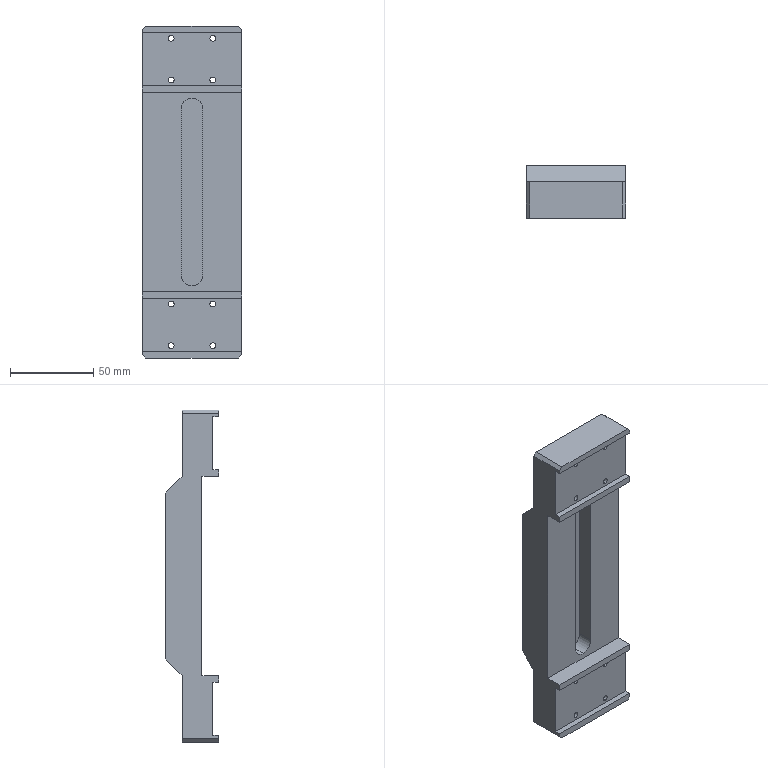Part | NX | features BREP 1 | 1 solid | 88 faces | box 60 x 32 x 200 mm | volume 228373 mm3 | cylinder 43 | plane 37 | cone 8 | commonest cylinder face diameters 3.4 x16 6 x16 2.5 x4 3.3 x4 13 x3